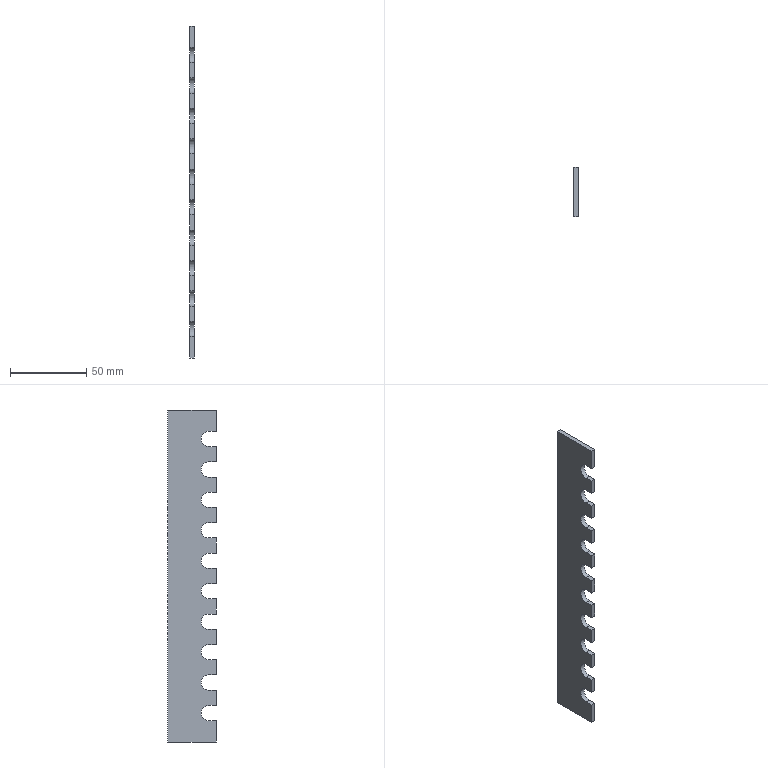Part | SolidWorks | features ExtruThin 1, ICE 1, LPattern 1 | 1 solid | 46 faces | box 3 x 32 x 218 mm | volume 18250 mm3 | plane 36 | cylinder 10 | commonest cylinder face diameters 10 x10
STEP:
#1=CARTESIAN_POINT('',(-3.,-32.,14.));
#2=VERTEX_POINT('',#1);
#3=CARTESIAN_POINT('',(0.,-32.,14.));
#4=VERTEX_POINT('',#3);
#5=CARTESIAN_POINT('',(-3.,-32.,14.));
#6=DIRECTION('',(1.,0.,0.));
#7=VECTOR('',#6,1000.);
#8=LINE('',#5,#7);
#9=EDGE_CURVE('',#2,#4,#8,.T.);
#10=ORIENTED_EDGE('',*,*,#9,.F.);
#11=CARTESIAN_POINT('',(-3.,-32.,0.));
#12=VERTEX_POINT('',#11);
#13=CARTESIAN_POINT('',(-3.,-32.,218.));
#14=DIRECTION('',(0.,0.,-1.));
#15=VECTOR('',#14,1000.);
#16=LINE('',#13,#15);
#17=EDGE_CURVE('',#2,#12,#16,.T.);
#18=ORIENTED_EDGE('',*,*,#17,.T.);
#19=CARTESIAN_POINT('',(0.,-32.,0.));
#20=VERTEX_POINT('',#19);
#21=CARTESIAN_POINT('',(0.,-32.,0.));
#22=DIRECTION('',(-1.,0.,0.));
#23=VECTOR('',#22,1000.);
#24=LINE('',#21,#23);
#25=EDGE_CURVE('',#20,#12,#24,.T.);
#26=ORIENTED_EDGE('',*,*,#25,.F.);
#27=CARTESIAN_POINT('',(0.,-32.,218.));
#28=DIRECTION('',(0.,0.,-1.));
#29=VECTOR('',#28,1000.);
#30=LINE('',#27,#29);
#31=EDGE_CURVE('',#4,#20,#30,.T.);
#32=ORIENTED_EDGE('',*,*,#31,.F.);
#33=EDGE_LOOP('',(#10,#18,#26,#32));
#34=FACE_OUTER_BOUND('',#33,.T.);
#35=CARTESIAN_POINT('',(0.,-32.,218.));
#36=DIRECTION('',(0.,-1.,0.));
#37=DIRECTION('',(0.,0.,-1.));
#38=AXIS2_PLACEMENT_3D('',#35,#36,#37);
#39=PLANE('',#38);
#40=ADVANCED_FACE('',(#34),#39,.T.);
#41=CARTESIAN_POINT('',(-3.,-32.,24.));
#42=VERTEX_POINT('',#41);
#43=CARTESIAN_POINT('',(0.,-32.,24.));
#44=VERTEX_POINT('',#43);
#45=CARTESIAN_POINT('',(-3.,-32.,24.));
#46=DIRECTION('',(1.,0.,0.));
#47=VECTOR('',#46,1000.);
#48=LINE('',#45,#47);
#49=EDGE_CURVE('',#42,#44,#48,.T.);
#50=ORIENTED_EDGE('',*,*,#49,.T.);
#51=CARTESIAN_POINT('',(0.,-32.,34.));
#52=VERTEX_POINT('',#51);
#53=CARTESIAN_POINT('',(0.,-32.,218.));
#54=DIRECTION('',(0.,0.,-1.));
#55=VECTOR('',#54,1000.);
#56=LINE('',#53,#55);
#57=EDGE_CURVE('',#52,#44,#56,.T.);
#58=ORIENTED_EDGE('',*,*,#57,.F.);
#59=CARTESIAN_POINT('',(-3.,-32.,34.));
#60=VERTEX_POINT('',#59);
#61=CARTESIAN_POINT('',(-3.,-32.,34.));
#62=DIRECTION('',(1.,0.,0.));
#63=VECTOR('',#62,1000.);
#64=LINE('',#61,#63);
#65=EDGE_CURVE('',#60,#52,#64,.T.);
#66=ORIENTED_EDGE('',*,*,#65,.F.);
#67=CARTESIAN_POINT('',(-3.,-32.,218.));
#68=DIRECTION('',(0.,0.,-1.));
#69=VECTOR('',#68,1000.);
#70=LINE('',#67,#69);
#71=EDGE_CURVE('',#60,#42,#70,.T.);
#72=ORIENTED_EDGE('',*,*,#71,.T.);
#73=EDGE_LOOP('',(#50,#58,#66,#72));
#74=FACE_OUTER_BOUND('',#73,.T.);
#75=CARTESIAN_POINT('',(0.,-32.,218.));
#76=DIRECTION('',(0.,-1.,0.));
#77=DIRECTION('',(0.,0.,-1.));
#78=AXIS2_PLACEMENT_3D('',#75,#76,#77);
#79=PLANE('',#78);
#80=ADVANCED_FACE('',(#74),#79,.T.);
#81=CARTESIAN_POINT('',(-3.,-32.,44.));
#82=VERTEX_POINT('',#81);
#83=CARTESIAN_POINT('',(0.,-32.,44.));
#84=VERTEX_POINT('',#83);
#85=CARTESIAN_POINT('',(-3.,-32.,44.));
#86=DIRECTION('',(1.,0.,0.));
#87=VECTOR('',#86,1000.);
#88=LINE('',#85,#87);
#89=EDGE_CURVE('',#82,#84,#88,.T.);
#90=ORIENTED_EDGE('',*,*,#89,.T.);
#91=CARTESIAN_POINT('',(0.,-32.,54.));
#92=VERTEX_POINT('',#91);
#93=CARTESIAN_POINT('',(0.,-32.,218.));
#94=DIRECTION('',(0.,0.,-1.));
#95=VECTOR('',#94,1000.);
#96=LINE('',#93,#95);
#97=EDGE_CURVE('',#92,#84,#96,.T.);
#98=ORIENTED_EDGE('',*,*,#97,.F.);
#99=CARTESIAN_POINT('',(-3.,-32.,54.));
#100=VERTEX_POINT('',#99);
#101=CARTESIAN_POINT('',(-3.,-32.,54.));
#102=DIRECTION('',(1.,0.,0.));
#103=VECTOR('',#102,1000.);
#104=LINE('',#101,#103);
#105=EDGE_CURVE('',#100,#92,#104,.T.);
#106=ORIENTED_EDGE('',*,*,#105,.F.);
#107=CARTESIAN_POINT('',(-3.,-32.,218.));
#108=DIRECTION('',(0.,0.,-1.));
#109=VECTOR('',#108,1000.);
#110=LINE('',#107,#109);
#111=EDGE_CURVE('',#100,#82,#110,.T.);
#112=ORIENTED_EDGE('',*,*,#111,.T.);
#113=EDGE_LOOP('',(#90,#98,#106,#112));
#114=FACE_OUTER_BOUND('',#113,.T.);
#115=CARTESIAN_POINT('',(0.,-32.,218.));
#116=DIRECTION('',(0.,-1.,0.));
#117=DIRECTION('',(0.,0.,-1.));
#118=AXIS2_PLACEMENT_3D('',#115,#116,#117);
#119=PLANE('',#118);
#120=ADVANCED_FACE('',(#114),#119,.T.);
#121=CARTESIAN_POINT('',(-3.,-32.,64.));
#122=VERTEX_POINT('',#121);
#123=CARTESIAN_POINT('',(0.,-32.,64.));
#124=VERTEX_POINT('',#123);
#125=CARTESIAN_POINT('',(-3.,-32.,64.));
#126=DIRECTION('',(1.,0.,0.));
#127=VECTOR('',#126,1000.);
#128=LINE('',#125,#127);
#129=EDGE_CURVE('',#122,#124,#128,.T.);
#130=ORIENTED_EDGE('',*,*,#129,.T.);
#131=CARTESIAN_POINT('',(0.,-32.,74.));
#132=VERTEX_POINT('',#131);
#133=CARTESIAN_POINT('',(0.,-32.,218.));
#134=DIRECTION('',(0.,0.,-1.));
#135=VECTOR('',#134,1000.);
#136=LINE('',#133,#135);
#137=EDGE_CURVE('',#132,#124,#136,.T.);
#138=ORIENTED_EDGE('',*,*,#137,.F.);
#139=CARTESIAN_POINT('',(-3.,-32.,74.));
#140=VERTEX_POINT('',#139);
#141=CARTESIAN_POINT('',(-3.,-32.,74.));
#142=DIRECTION('',(1.,0.,0.));
#143=VECTOR('',#142,1000.);
#144=LINE('',#141,#143);
#145=EDGE_CURVE('',#140,#132,#144,.T.);
#146=ORIENTED_EDGE('',*,*,#145,.F.);
#147=CARTESIAN_POINT('',(-3.,-32.,218.));
#148=DIRECTION('',(0.,0.,-1.));
#149=VECTOR('',#148,1000.);
#150=LINE('',#147,#149);
#151=EDGE_CURVE('',#140,#122,#150,.T.);
#152=ORIENTED_EDGE('',*,*,#151,.T.);
#153=EDGE_LOOP('',(#130,#138,#146,#152));
#154=FACE_OUTER_BOUND('',#153,.T.);
#155=CARTESIAN_POINT('',(0.,-32.,218.));
#156=DIRECTION('',(0.,-1.,0.));
#157=DIRECTION('',(0.,0.,-1.));
#158=AXIS2_PLACEMENT_3D('',#155,#156,#157);
#159=PLANE('',#158);
#160=ADVANCED_FACE('',(#154),#159,.T.);
#161=CARTESIAN_POINT('',(-3.,-32.,84.));
#162=VERTEX_POINT('',#161);
#163=CARTESIAN_POINT('',(0.,-32.,84.));
#164=VERTEX_POINT('',#163);
#165=CARTESIAN_POINT('',(-3.,-32.,84.));
#166=DIRECTION('',(1.,0.,0.));
#167=VECTOR('',#166,1000.);
#168=LINE('',#165,#167);
#169=EDGE_CURVE('',#162,#164,#168,.T.);
#170=ORIENTED_EDGE('',*,*,#169,.T.);
#171=CARTESIAN_POINT('',(0.,-32.,94.));
#172=VERTEX_POINT('',#171);
#173=CARTESIAN_POINT('',(0.,-32.,218.));
#174=DIRECTION('',(0.,0.,-1.));
#175=VECTOR('',#174,1000.);
#176=LINE('',#173,#175);
#177=EDGE_CURVE('',#172,#164,#176,.T.);
#178=ORIENTED_EDGE('',*,*,#177,.F.);
#179=CARTESIAN_POINT('',(-3.,-32.,94.));
#180=VERTEX_POINT('',#179);
#181=CARTESIAN_POINT('',(-3.,-32.,94.));
#182=DIRECTION('',(1.,0.,0.));
#183=VECTOR('',#182,1000.);
#184=LINE('',#181,#183);
#185=EDGE_CURVE('',#180,#172,#184,.T.);
#186=ORIENTED_EDGE('',*,*,#185,.F.);
#187=CARTESIAN_POINT('',(-3.,-32.,218.));
#188=DIRECTION('',(0.,0.,-1.));
#189=VECTOR('',#188,1000.);
#190=LINE('',#187,#189);
#191=EDGE_CURVE('',#180,#162,#190,.T.);
#192=ORIENTED_EDGE('',*,*,#191,.T.);
#193=EDGE_LOOP('',(#170,#178,#186,#192));
#194=FACE_OUTER_BOUND('',#193,.T.);
#195=CARTESIAN_POINT('',(0.,-32.,218.));
#196=DIRECTION('',(0.,-1.,0.));
#197=DIRECTION('',(0.,0.,-1.));
#198=AXIS2_PLACEMENT_3D('',#195,#196,#197);
#199=PLANE('',#198);
#200=ADVANCED_FACE('',(#194),#199,.T.);
#201=CARTESIAN_POINT('',(-3.,-32.,104.));
#202=VERTEX_POINT('',#201);
#203=CARTESIAN_POINT('',(0.,-32.,104.));
#204=VERTEX_POINT('',#203);
#205=CARTESIAN_POINT('',(-3.,-32.,104.));
#206=DIRECTION('',(1.,0.,0.));
#207=VECTOR('',#206,1000.);
#208=LINE('',#205,#207);
#209=EDGE_CURVE('',#202,#204,#208,.T.);
#210=ORIENTED_EDGE('',*,*,#209,.T.);
#211=CARTESIAN_POINT('',(0.,-32.,114.));
#212=VERTEX_POINT('',#211);
#213=CARTESIAN_POINT('',(0.,-32.,218.));
#214=DIRECTION('',(0.,0.,-1.));
#215=VECTOR('',#214,1000.);
#216=LINE('',#213,#215);
#217=EDGE_CURVE('',#212,#204,#216,.T.);
#218=ORIENTED_EDGE('',*,*,#217,.F.);
#219=CARTESIAN_POINT('',(-3.,-32.,114.));
#220=VERTEX_POINT('',#219);
#221=CARTESIAN_POINT('',(-3.,-32.,114.));
#222=DIRECTION('',(1.,0.,0.));
#223=VECTOR('',#222,1000.);
#224=LINE('',#221,#223);
#225=EDGE_CURVE('',#220,#212,#224,.T.);
#226=ORIENTED_EDGE('',*,*,#225,.F.);
#227=CARTESIAN_POINT('',(-3.,-32.,218.));
#228=DIRECTION('',(0.,0.,-1.));
#229=VECTOR('',#228,1000.);
#230=LINE('',#227,#229);
#231=EDGE_CURVE('',#220,#202,#230,.T.);
#232=ORIENTED_EDGE('',*,*,#231,.T.);
#233=EDGE_LOOP('',(#210,#218,#226,#232));
#234=FACE_OUTER_BOUND('',#233,.T.);
#235=CARTESIAN_POINT('',(0.,-32.,218.));
#236=DIRECTION('',(0.,-1.,0.));
#237=DIRECTION('',(0.,0.,-1.));
#238=AXIS2_PLACEMENT_3D('',#235,#236,#237);
#239=PLANE('',#238);
#240=ADVANCED_FACE('',(#234),#239,.T.);
#241=CARTESIAN_POINT('',(-3.,-32.,124.));
#242=VERTEX_POINT('',#241);
#243=CARTESIAN_POINT('',(0.,-32.,124.));
#244=VERTEX_POINT('',#243);
#245=CARTESIAN_POINT('',(-3.,-32.,124.));
#246=DIRECTION('',(1.,0.,0.));
#247=VECTOR('',#246,1000.);
#248=LINE('',#245,#247);
#249=EDGE_CURVE('',#242,#244,#248,.T.);
#250=ORIENTED_EDGE('',*,*,#249,.T.);
#251=CARTESIAN_POINT('',(0.,-32.,134.));
#252=VERTEX_POINT('',#251);
#253=CARTESIAN_POINT('',(0.,-32.,218.));
#254=DIRECTION('',(0.,0.,-1.));
#255=VECTOR('',#254,1000.);
#256=LINE('',#253,#255);
#257=EDGE_CURVE('',#252,#244,#256,.T.);
#258=ORIENTED_EDGE('',*,*,#257,.F.);
#259=CARTESIAN_POINT('',(-3.,-32.,134.));
#260=VERTEX_POINT('',#259);
#261=CARTESIAN_POINT('',(-3.,-32.,134.));
#262=DIRECTION('',(1.,0.,0.));
#263=VECTOR('',#262,1000.);
#264=LINE('',#261,#263);
#265=EDGE_CURVE('',#260,#252,#264,.T.);
#266=ORIENTED_EDGE('',*,*,#265,.F.);
#267=CARTESIAN_POINT('',(-3.,-32.,218.));
#268=DIRECTION('',(0.,0.,-1.));
#269=VECTOR('',#268,1000.);
#270=LINE('',#267,#269);
#271=EDGE_CURVE('',#260,#242,#270,.T.);
#272=ORIENTED_EDGE('',*,*,#271,.T.);
#273=EDGE_LOOP('',(#250,#258,#266,#272));
#274=FACE_OUTER_BOUND('',#273,.T.);
#275=CARTESIAN_POINT('',(0.,-32.,218.));
#276=DIRECTION('',(0.,-1.,0.));
#277=DIRECTION('',(0.,0.,-1.));
#278=AXIS2_PLACEMENT_3D('',#275,#276,#277);
#279=PLANE('',#278);
#280=ADVANCED_FACE('',(#274),#279,.T.);
#281=CARTESIAN_POINT('',(-3.,-32.,144.));
#282=VERTEX_POINT('',#281);
#283=CARTESIAN_POINT('',(0.,-32.,144.));
#284=VERTEX_POINT('',#283);
#285=CARTESIAN_POINT('',(-3.,-32.,144.));
#286=DIRECTION('',(1.,0.,0.));
#287=VECTOR('',#286,1000.);
#288=LINE('',#285,#287);
#289=EDGE_CURVE('',#282,#284,#288,.T.);
#290=ORIENTED_EDGE('',*,*,#289,.T.);
#291=CARTESIAN_POINT('',(0.,-32.,154.));
#292=VERTEX_POINT('',#291);
#293=CARTESIAN_POINT('',(0.,-32.,218.));
#294=DIRECTION('',(0.,0.,-1.));
#295=VECTOR('',#294,1000.);
#296=LINE('',#293,#295);
#297=EDGE_CURVE('',#292,#284,#296,.T.);
#298=ORIENTED_EDGE('',*,*,#297,.F.);
#299=CARTESIAN_POINT('',(-3.,-32.,154.));
#300=VERTEX_POINT('',#299);
#301=CARTESIAN_POINT('',(-3.,-32.,154.));
#302=DIRECTION('',(1.,0.,0.));
#303=VECTOR('',#302,1000.);
#304=LINE('',#301,#303);
#305=EDGE_CURVE('',#300,#292,#304,.T.);
#306=ORIENTED_EDGE('',*,*,#305,.F.);
#307=CARTESIAN_POINT('',(-3.,-32.,218.));
#308=DIRECTION('',(0.,0.,-1.));
#309=VECTOR('',#308,1000.);
#310=LINE('',#307,#309);
#311=EDGE_CURVE('',#300,#282,#310,.T.);
#312=ORIENTED_EDGE('',*,*,#311,.T.);
#313=EDGE_LOOP('',(#290,#298,#306,#312));
#314=FACE_OUTER_BOUND('',#313,.T.);
#315=CARTESIAN_POINT('',(0.,-32.,218.));
#316=DIRECTION('',(0.,-1.,0.));
#317=DIRECTION('',(0.,0.,-1.));
#318=AXIS2_PLACEMENT_3D('',#315,#316,#317);
#319=PLANE('',#318);
#320=ADVANCED_FACE('',(#314),#319,.T.);
#321=CARTESIAN_POINT('',(-3.,-32.,164.));
#322=VERTEX_POINT('',#321);
#323=CARTESIAN_POINT('',(0.,-32.,164.));
#324=VERTEX_POINT('',#323);
#325=CARTESIAN_POINT('',(-3.,-32.,164.));
#326=DIRECTION('',(1.,0.,0.));
#327=VECTOR('',#326,1000.);
#328=LINE('',#325,#327);
#329=EDGE_CURVE('',#322,#324,#328,.T.);
#330=ORIENTED_EDGE('',*,*,#329,.T.);
#331=CARTESIAN_POINT('',(0.,-32.,174.));
#332=VERTEX_POINT('',#331);
#333=CARTESIAN_POINT('',(0.,-32.,218.));
#334=DIRECTION('',(0.,0.,-1.));
#335=VECTOR('',#334,1000.);
#336=LINE('',#333,#335);
#337=EDGE_CURVE('',#332,#324,#336,.T.);
#338=ORIENTED_EDGE('',*,*,#337,.F.);
#339=CARTESIAN_POINT('',(-3.,-32.,174.));
#340=VERTEX_POINT('',#339);
#341=CARTESIAN_POINT('',(-3.,-32.,174.));
#342=DIRECTION('',(1.,0.,0.));
#343=VECTOR('',#342,1000.);
#344=LINE('',#341,#343);
#345=EDGE_CURVE('',#340,#332,#344,.T.);
#346=ORIENTED_EDGE('',*,*,#345,.F.);
#347=CARTESIAN_POINT('',(-3.,-32.,218.));
#348=DIRECTION('',(0.,0.,-1.));
#349=VECTOR('',#348,1000.);
#350=LINE('',#347,#349);
#351=EDGE_CURVE('',#340,#322,#350,.T.);
#352=ORIENTED_EDGE('',*,*,#351,.T.);
#353=EDGE_LOOP('',(#330,#338,#346,#352));
#354=FACE_OUTER_BOUND('',#353,.T.);
#355=CARTESIAN_POINT('',(0.,-32.,218.));
#356=DIRECTION('',(0.,-1.,0.));
#357=DIRECTION('',(0.,0.,-1.));
#358=AXIS2_PLACEMENT_3D('',#355,#356,#357);
#359=PLANE('',#358);
#360=ADVANCED_FACE('',(#354),#359,.T.);
#361=CARTESIAN_POINT('',(-3.,-32.,184.));
#362=VERTEX_POINT('',#361);
#363=CARTESIAN_POINT('',(0.,-32.,184.));
#364=VERTEX_POINT('',#363);
#365=CARTESIAN_POINT('',(-3.,-32.,184.));
#366=DIRECTION('',(1.,0.,0.));
#367=VECTOR('',#366,1000.);
#368=LINE('',#365,#367);
#369=EDGE_CURVE('',#362,#364,#368,.T.);
#370=ORIENTED_EDGE('',*,*,#369,.T.);
#371=CARTESIAN_POINT('',(0.,-32.,194.));
#372=VERTEX_POINT('',#371);
#373=CARTESIAN_POINT('',(0.,-32.,218.));
#374=DIRECTION('',(0.,0.,-1.));
#375=VECTOR('',#374,1000.);
#376=LINE('',#373,#375);
#377=EDGE_CURVE('',#372,#364,#376,.T.);
#378=ORIENTED_EDGE('',*,*,#377,.F.);
#379=CARTESIAN_POINT('',(-3.,-32.,194.));
#380=VERTEX_POINT('',#379);
#381=CARTESIAN_POINT('',(-3.,-32.,194.));
#382=DIRECTION('',(1.,0.,0.));
#383=VECTOR('',#382,1000.);
#384=LINE('',#381,#383);
#385=EDGE_CURVE('',#380,#372,#384,.T.);
#386=ORIENTED_EDGE('',*,*,#385,.F.);
#387=CARTESIAN_POINT('',(-3.,-32.,218.));
#388=DIRECTION('',(0.,0.,-1.));
#389=VECTOR('',#388,1000.);
#390=LINE('',#387,#389);
#391=EDGE_CURVE('',#380,#362,#390,.T.);
#392=ORIENTED_EDGE('',*,*,#391,.T.);
#393=EDGE_LOOP('',(#370,#378,#386,#392));
#394=FACE_OUTER_BOUND('',#393,.T.);
#395=CARTESIAN_POINT('',(0.,-32.,218.));
#396=DIRECTION('',(0.,-1.,0.));
#397=DIRECTION('',(0.,0.,-1.));
#398=AXIS2_PLACEMENT_3D('',#395,#396,#397);
#399=PLANE('',#398);
#400=ADVANCED_FACE('',(#394),#399,.T.);
#401=ORIENTED_EDGE('',*,*,#17,.F.);
#402=CARTESIAN_POINT('',(-3.,-27.,14.));
#403=VERTEX_POINT('',#402);
#404=CARTESIAN_POINT('',(-3.,-27.,14.));
#405=DIRECTION('',(0.,1.,0.));
#406=VECTOR('',#405,1000.);
#407=LINE('',#404,#406);
#408=EDGE_CURVE('',#2,#403,#407,.T.);
#409=ORIENTED_EDGE('',*,*,#408,.T.);
#410=CARTESIAN_POINT('',(-3.,-27.,24.));
#411=VERTEX_POINT('',#410);
#412=CARTESIAN_POINT('',(-3.,-27.,19.));
#413=DIRECTION('',(1.,0.,0.));
#414=DIRECTION('',(0.,0.,-1.));
#415=AXIS2_PLACEMENT_3D('',#412,#413,#414);
#416=CIRCLE('',#415,5.);
#417=EDGE_CURVE('',#403,#411,#416,.T.);
#418=ORIENTED_EDGE('',*,*,#417,.T.);
#419=CARTESIAN_POINT('',(-3.,-32.,24.));
#420=DIRECTION('',(0.,-1.,0.));
#421=VECTOR('',#420,1000.);
#422=LINE('',#419,#421);
#423=EDGE_CURVE('',#411,#42,#422,.T.);
#424=ORIENTED_EDGE('',*,*,#423,.T.);
#425=ORIENTED_EDGE('',*,*,#71,.F.);
#426=CARTESIAN_POINT('',(-3.,-27.,34.));
#427=VERTEX_POINT('',#426);
#428=CARTESIAN_POINT('',(-3.,-27.,34.));
#429=DIRECTION('',(0.,1.,0.));
#430=VECTOR('',#429,1000.);
#431=LINE('',#428,#430);
#432=EDGE_CURVE('',#60,#427,#431,.T.);
#433=ORIENTED_EDGE('',*,*,#432,.T.);
#434=CARTESIAN_POINT('',(-3.,-27.,44.));
#435=VERTEX_POINT('',#434);
#436=CARTESIAN_POINT('',(-3.,-27.,39.));
#437=DIRECTION('',(1.,0.,0.));
#438=DIRECTION('',(0.,0.,-1.));
#439=AXIS2_PLACEMENT_3D('',#436,#437,#438);
#440=CIRCLE('',#439,5.);
#441=EDGE_CURVE('',#427,#435,#440,.T.);
#442=ORIENTED_EDGE('',*,*,#441,.T.);
#443=CARTESIAN_POINT('',(-3.,-32.,44.));
#444=DIRECTION('',(0.,-1.,0.));
#445=VECTOR('',#444,1000.);
#446=LINE('',#443,#445);
#447=EDGE_CURVE('',#435,#82,#446,.T.);
#448=ORIENTED_EDGE('',*,*,#447,.T.);
#449=ORIENTED_EDGE('',*,*,#111,.F.);
#450=CARTESIAN_POINT('',(-3.,-27.,54.));
#451=VERTEX_POINT('',#450);
#452=CARTESIAN_POINT('',(-3.,-27.,54.));
#453=DIRECTION('',(0.,1.,0.));
#454=VECTOR('',#453,1000.);
#455=LINE('',#452,#454);
#456=EDGE_CURVE('',#100,#451,#455,.T.);
#457=ORIENTED_EDGE('',*,*,#456,.T.);
#458=CARTESIAN_POINT('',(-3.,-27.,64.));
#459=VERTEX_POINT('',#458);
#460=CARTESIAN_POINT('',(-3.,-27.,59.));
#461=DIRECTION('',(1.,0.,0.));
#462=DIRECTION('',(0.,0.,-1.));
#463=AXIS2_PLACEMENT_3D('',#460,#461,#462);
#464=CIRCLE('',#463,5.);
#465=EDGE_CURVE('',#451,#459,#464,.T.);
#466=ORIENTED_EDGE('',*,*,#465,.T.);
#467=CARTESIAN_POINT('',(-3.,-32.,64.));
#468=DIRECTION('',(0.,-1.,0.));
#469=VECTOR('',#468,1000.);
#470=LINE('',#467,#469);
#471=EDGE_CURVE('',#459,#122,#470,.T.);
#472=ORIENTED_EDGE('',*,*,#471,.T.);
#473=ORIENTED_EDGE('',*,*,#151,.F.);
#474=CARTESIAN_POINT('',(-3.,-27.,74.));
#475=VERTEX_POINT('',#474);
#476=CARTESIAN_POINT('',(-3.,-27.,74.));
#477=DIRECTION('',(0.,1.,0.));
#478=VECTOR('',#477,1000.);
#479=LINE('',#476,#478);
#480=EDGE_CURVE('',#140,#475,#479,.T.);
#481=ORIENTED_EDGE('',*,*,#480,.T.);
#482=CARTESIAN_POINT('',(-3.,-27.,84.));
#483=VERTEX_POINT('',#482);
#484=CARTESIAN_POINT('',(-3.,-27.,79.));
#485=DIRECTION('',(1.,0.,0.));
#486=DIRECTION('',(0.,0.,-1.));
#487=AXIS2_PLACEMENT_3D('',#484,#485,#486);
#488=CIRCLE('',#487,5.);
#489=EDGE_CURVE('',#475,#483,#488,.T.);
#490=ORIENTED_EDGE('',*,*,#489,.T.);
#491=CARTESIAN_POINT('',(-3.,-32.,84.));
#492=DIRECTION('',(0.,-1.,0.));
#493=VECTOR('',#492,1000.);
#494=LINE('',#491,#493);
#495=EDGE_CURVE('',#483,#162,#494,.T.);
#496=ORIENTED_EDGE('',*,*,#495,.T.);
#497=ORIENTED_EDGE('',*,*,#191,.F.);
#498=CARTESIAN_POINT('',(-3.,-27.,94.));
#499=VERTEX_POINT('',#498);
#500=CARTESIAN_POINT('',(-3.,-27.,94.));
#501=DIRECTION('',(0.,1.,0.));
#502=VECTOR('',#501,1000.);
#503=LINE('',#500,#502);
#504=EDGE_CURVE('',#180,#499,#503,.T.);
#505=ORIENTED_EDGE('',*,*,#504,.T.);
#506=CARTESIAN_POINT('',(-3.,-27.,104.));
#507=VERTEX_POINT('',#506);
#508=CARTESIAN_POINT('',(-3.,-27.,99.));
#509=DIRECTION('',(1.,0.,0.));
#510=DIRECTION('',(0.,0.,-1.));
#511=AXIS2_PLACEMENT_3D('',#508,#509,#510);
#512=CIRCLE('',#511,5.);
#513=EDGE_CURVE('',#499,#507,#512,.T.);
#514=ORIENTED_EDGE('',*,*,#513,.T.);
#515=CARTESIAN_POINT('',(-3.,-32.,104.));
#516=DIRECTION('',(0.,-1.,0.));
#517=VECTOR('',#516,1000.);
#518=LINE('',#515,#517);
#519=EDGE_CURVE('',#507,#202,#518,.T.);
#520=ORIENTED_EDGE('',*,*,#519,.T.);
#521=ORIENTED_EDGE('',*,*,#231,.F.);
#522=CARTESIAN_POINT('',(-3.,-27.,114.));
#523=VERTEX_POINT('',#522);
#524=CARTESIAN_POINT('',(-3.,-27.,114.));
#525=DIRECTION('',(0.,1.,0.));
#526=VECTOR('',#525,1000.);
#527=LINE('',#524,#526);
#528=EDGE_CURVE('',#220,#523,#527,.T.);
#529=ORIENTED_EDGE('',*,*,#528,.T.);
#530=CARTESIAN_POINT('',(-3.,-27.,124.));
#531=VERTEX_POINT('',#530);
#532=CARTESIAN_POINT('',(-3.,-27.,119.));
#533=DIRECTION('',(1.,0.,0.));
#534=DIRECTION('',(0.,0.,-1.));
#535=AXIS2_PLACEMENT_3D('',#532,#533,#534);
#536=CIRCLE('',#535,5.);
#537=EDGE_CURVE('',#523,#531,#536,.T.);
#538=ORIENTED_EDGE('',*,*,#537,.T.);
#539=CARTESIAN_POINT('',(-3.,-32.,124.));
#540=DIRECTION('',(0.,-1.,0.));
#541=VECTOR('',#540,1000.);
#542=LINE('',#539,#541);
#543=EDGE_CURVE('',#531,#242,#542,.T.);
#544=ORIENTED_EDGE('',*,*,#543,.T.);
#545=ORIENTED_EDGE('',*,*,#271,.F.);
#546=CARTESIAN_POINT('',(-3.,-27.,134.));
#547=VERTEX_POINT('',#546);
#548=CARTESIAN_POINT('',(-3.,-27.,134.));
#549=DIRECTION('',(0.,1.,0.));
#550=VECTOR('',#549,1000.);
#551=LINE('',#548,#550);
#552=EDGE_CURVE('',#260,#547,#551,.T.);
#553=ORIENTED_EDGE('',*,*,#552,.T.);
#554=CARTESIAN_POINT('',(-3.,-27.,144.));
#555=VERTEX_POINT('',#554);
#556=CARTESIAN_POINT('',(-3.,-27.,139.));
#557=DIRECTION('',(1.,0.,0.));
#558=DIRECTION('',(0.,0.,-1.));
#559=AXIS2_PLACEMENT_3D('',#556,#557,#558);
#560=CIRCLE('',#559,5.);
#561=EDGE_CURVE('',#547,#555,#560,.T.);
#562=ORIENTED_EDGE('',*,*,#561,.T.);
#563=CARTESIAN_POINT('',(-3.,-32.,144.));
#564=DIRECTION('',(0.,-1.,0.));
#565=VECTOR('',#564,1000.);
#566=LINE('',#563,#565);
#567=EDGE_CURVE('',#555,#282,#566,.T.);
#568=ORIENTED_EDGE('',*,*,#567,.T.);
#569=ORIENTED_EDGE('',*,*,#311,.F.);
#570=CARTESIAN_POINT('',(-3.,-27.,154.));
#571=VERTEX_POINT('',#570);
#572=CARTESIAN_POINT('',(-3.,-27.,154.));
#573=DIRECTION('',(0.,1.,0.));
#574=VECTOR('',#573,1000.);
#575=LINE('',#572,#574);
#576=EDGE_CURVE('',#300,#571,#575,.T.);
#577=ORIENTED_EDGE('',*,*,#576,.T.);
#578=CARTESIAN_POINT('',(-3.,-27.,164.));
#579=VERTEX_POINT('',#578);
#580=CARTESIAN_POINT('',(-3.,-27.,159.));
#581=DIRECTION('',(1.,0.,0.));
#582=DIRECTION('',(0.,0.,-1.));
#583=AXIS2_PLACEMENT_3D('',#580,#581,#582);
#584=CIRCLE('',#583,5.);
#585=EDGE_CURVE('',#571,#579,#584,.T.);
#586=ORIENTED_EDGE('',*,*,#585,.T.);
#587=CARTESIAN_POINT('',(-3.,-32.,164.));
#588=DIRECTION('',(0.,-1.,0.));
#589=VECTOR('',#588,1000.);
#590=LINE('',#587,#589);
#591=EDGE_CURVE('',#579,#322,#590,.T.);
#592=ORIENTED_EDGE('',*,*,#591,.T.);
#593=ORIENTED_EDGE('',*,*,#351,.F.);
#594=CARTESIAN_POINT('',(-3.,-27.,174.));
#595=VERTEX_POINT('',#594);
#596=CARTESIAN_POINT('',(-3.,-27.,174.));
#597=DIRECTION('',(0.,1.,0.));
#598=VECTOR('',#597,1000.);
#599=LINE('',#596,#598);
#600=EDGE_CURVE('',#340,#595,#599,.T.);
#601=ORIENTED_EDGE('',*,*,#600,.T.);
#602=CARTESIAN_POINT('',(-3.,-27.,184.));
#603=VERTEX_POINT('',#602);
#604=CARTESIAN_POINT('',(-3.,-27.,179.));
#605=DIRECTION('',(1.,0.,0.));
#606=DIRECTION('',(0.,0.,-1.));
#607=AXIS2_PLACEMENT_3D('',#604,#605,#606);
#608=CIRCLE('',#607,5.);
#609=EDGE_CURVE('',#595,#603,#608,.T.);
#610=ORIENTED_EDGE('',*,*,#609,.T.);
#611=CARTESIAN_POINT('',(-3.,-32.,184.));
#612=DIRECTION('',(0.,-1.,0.));
#613=VECTOR('',#612,1000.);
#614=LINE('',#611,#613);
#615=EDGE_CURVE('',#603,#362,#614,.T.);
#616=ORIENTED_EDGE('',*,*,#615,.T.);
#617=ORIENTED_EDGE('',*,*,#391,.F.);
#618=CARTESIAN_POINT('',(-3.,-27.,194.));
#619=VERTEX_POINT('',#618);
#620=CARTESIAN_POINT('',(-3.,-27.,194.));
#621=DIRECTION('',(0.,1.,0.));
#622=VECTOR('',#621,1000.);
#623=LINE('',#620,#622);
#624=EDGE_CURVE('',#380,#619,#623,.T.);
#625=ORIENTED_EDGE('',*,*,#624,.T.);
#626=CARTESIAN_POINT('',(-3.,-27.,204.));
#627=VERTEX_POINT('',#626);
#628=CARTESIAN_POINT('',(-3.,-27.,199.));
#629=DIRECTION('',(1.,0.,0.));
#630=DIRECTION('',(0.,0.,-1.));
#631=AXIS2_PLACEMENT_3D('',#628,#629,#630);
#632=CIRCLE('',#631,5.);
#633=EDGE_CURVE('',#619,#627,#632,.T.);
#634=ORIENTED_EDGE('',*,*,#633,.T.);
#635=CARTESIAN_POINT('',(-3.,-32.,204.));
#636=VERTEX_POINT('',#635);
#637=CARTESIAN_POINT('',(-3.,-32.,204.));
#638=DIRECTION('',(0.,-1.,0.));
#639=VECTOR('',#638,1000.);
#640=LINE('',#637,#639);
#641=EDGE_CURVE('',#627,#636,#640,.T.);
#642=ORIENTED_EDGE('',*,*,#641,.T.);
#643=CARTESIAN_POINT('',(-3.,-32.,218.));
#644=VERTEX_POINT('',#643);
#645=CARTESIAN_POINT('',(-3.,-32.,218.));
#646=DIRECTION('',(0.,0.,-1.));
#647=VECTOR('',#646,1000.);
#648=LINE('',#645,#647);
#649=EDGE_CURVE('',#644,#636,#648,.T.);
#650=ORIENTED_EDGE('',*,*,#649,.F.);
#651=CARTESIAN_POINT('',(-3.,0.,218.));
#652=VERTEX_POINT('',#651);
#653=CARTESIAN_POINT('',(-3.,0.,218.));
#654=DIRECTION('',(0.,-1.,0.));
#655=VECTOR('',#654,1000.);
#656=LINE('',#653,#655);
#657=EDGE_CURVE('',#652,#644,#656,.T.);
#658=ORIENTED_EDGE('',*,*,#657,.F.);
#659=CARTESIAN_POINT('',(-3.,0.,0.));
#660=VERTEX_POINT('',#659);
#661=CARTESIAN_POINT('',(-3.,0.,218.));
#662=DIRECTION('',(0.,0.,-1.));
#663=VECTOR('',#662,1000.);
#664=LINE('',#661,#663);
#665=EDGE_CURVE('',#652,#660,#664,.T.);
#666=ORIENTED_EDGE('',*,*,#665,.T.);
#667=CARTESIAN_POINT('',(-3.,0.,0.));
#668=DIRECTION('',(0.,-1.,0.));
#669=VECTOR('',#668,1000.);
#670=LINE('',#667,#669);
#671=EDGE_CURVE('',#660,#12,#670,.T.);
#672=ORIENTED_EDGE('',*,*,#671,.T.);
#673=EDGE_LOOP('',(#401,#409,#418,#424,#425,#433,#442,#448,#449,#457,#466,#472,#473,#481,#490,#496,#497,#505,#514,#520,#521,#529,#538,#544,#545,#553,#562,#568,#569,#577,#586,#592,#593,#601,#610,#616,#617,#625,#634,#642,#650,#658,#666,#672));
#674=FACE_OUTER_BOUND('',#673,.T.);
#675=CARTESIAN_POINT('',(-3.,0.,218.));
#676=DIRECTION('',(1.,0.,0.));
#677=DIRECTION('',(0.,1.,0.));
#678=AXIS2_PLACEMENT_3D('',#675,#676,#677);
#679=PLANE('',#678);
#680=ADVANCED_FACE('',(#674),#679,.F.);
#681=CARTESIAN_POINT('',(0.,-32.,204.));
#682=VERTEX_POINT('',#681);
#683=CARTESIAN_POINT('',(-3.,-32.,204.));
#684=DIRECTION('',(1.,0.,0.));
#685=VECTOR('',#684,1000.);
#686=LINE('',#683,#685);
#687=EDGE_CURVE('',#636,#682,#686,.T.);
#688=ORIENTED_EDGE('',*,*,#687,.T.);
#689=CARTESIAN_POINT('',(0.,-32.,218.));
#690=VERTEX_POINT('',#689);
#691=CARTESIAN_POINT('',(0.,-32.,218.));
#692=DIRECTION('',(0.,0.,-1.));
#693=VECTOR('',#692,1000.);
#694=LINE('',#691,#693);
#695=EDGE_CURVE('',#690,#682,#694,.T.);
#696=ORIENTED_EDGE('',*,*,#695,.F.);
#697=CARTESIAN_POINT('',(0.,-32.,218.));
#698=DIRECTION('',(-1.,0.,0.));
#699=VECTOR('',#698,1000.);
#700=LINE('',#697,#699);
#701=EDGE_CURVE('',#690,#644,#700,.T.);
#702=ORIENTED_EDGE('',*,*,#701,.T.);
#703=ORIENTED_EDGE('',*,*,#649,.T.);
#704=EDGE_LOOP('',(#688,#696,#702,#703));
#705=FACE_OUTER_BOUND('',#704,.T.);
#706=CARTESIAN_POINT('',(0.,-32.,218.));
#707=DIRECTION('',(0.,-1.,0.));
#708=DIRECTION('',(0.,0.,-1.));
#709=AXIS2_PLACEMENT_3D('',#706,#707,#708);
#710=PLANE('',#709);
#711=ADVANCED_FACE('',(#705),#710,.T.);
#712=CARTESIAN_POINT('',(0.,-27.,14.));
#713=VERTEX_POINT('',#712);
#714=CARTESIAN_POINT('',(0.,-27.,14.));
#715=DIRECTION('',(0.,1.,0.));
#716=VECTOR('',#715,1000.);
#717=LINE('',#714,#716);
#718=EDGE_CURVE('',#4,#713,#717,.T.);
#719=ORIENTED_EDGE('',*,*,#718,.F.);
#720=ORIENTED_EDGE('',*,*,#31,.T.);
#721=CARTESIAN_POINT('',(0.,0.,0.));
#722=VERTEX_POINT('',#721);
#723=CARTESIAN_POINT('',(0.,0.,0.));
#724=DIRECTION('',(0.,-1.,0.));
#725=VECTOR('',#724,1000.);
#726=LINE('',#723,#725);
#727=EDGE_CURVE('',#722,#20,#726,.T.);
#728=ORIENTED_EDGE('',*,*,#727,.F.);
#729=CARTESIAN_POINT('',(0.,0.,218.));
#730=VERTEX_POINT('',#729);
#731=CARTESIAN_POINT('',(0.,0.,218.));
#732=DIRECTION('',(0.,0.,-1.));
#733=VECTOR('',#732,1000.);
#734=LINE('',#731,#733);
#735=EDGE_CURVE('',#730,#722,#734,.T.);
#736=ORIENTED_EDGE('',*,*,#735,.F.);
#737=CARTESIAN_POINT('',(0.,0.,218.));
#738=DIRECTION('',(0.,-1.,0.));
#739=VECTOR('',#738,1000.);
#740=LINE('',#737,#739);
#741=EDGE_CURVE('',#730,#690,#740,.T.);
#742=ORIENTED_EDGE('',*,*,#741,.T.);
#743=ORIENTED_EDGE('',*,*,#695,.T.);
#744=CARTESIAN_POINT('',(0.,-27.,204.));
#745=VERTEX_POINT('',#744);
#746=CARTESIAN_POINT('',(0.,-32.,204.));
#747=DIRECTION('',(0.,-1.,0.));
#748=VECTOR('',#747,1000.);
#749=LINE('',#746,#748);
#750=EDGE_CURVE('',#745,#682,#749,.T.);
#751=ORIENTED_EDGE('',*,*,#750,.F.);
#752=CARTESIAN_POINT('',(0.,-27.,194.));
#753=VERTEX_POINT('',#752);
#754=CARTESIAN_POINT('',(0.,-27.,199.));
#755=DIRECTION('',(1.,0.,0.));
#756=DIRECTION('',(0.,0.,-1.));
#757=AXIS2_PLACEMENT_3D('',#754,#755,#756);
#758=CIRCLE('',#757,5.);
#759=EDGE_CURVE('',#753,#745,#758,.T.);
#760=ORIENTED_EDGE('',*,*,#759,.F.);
#761=CARTESIAN_POINT('',(0.,-27.,194.));
#762=DIRECTION('',(0.,1.,0.));
#763=VECTOR('',#762,1000.);
#764=LINE('',#761,#763);
#765=EDGE_CURVE('',#372,#753,#764,.T.);
#766=ORIENTED_EDGE('',*,*,#765,.F.);
#767=ORIENTED_EDGE('',*,*,#377,.T.);
#768=CARTESIAN_POINT('',(0.,-27.,184.));
#769=VERTEX_POINT('',#768);
#770=CARTESIAN_POINT('',(0.,-32.,184.));
#771=DIRECTION('',(0.,-1.,0.));
#772=VECTOR('',#771,1000.);
#773=LINE('',#770,#772);
#774=EDGE_CURVE('',#769,#364,#773,.T.);
#775=ORIENTED_EDGE('',*,*,#774,.F.);
#776=CARTESIAN_POINT('',(0.,-27.,174.));
#777=VERTEX_POINT('',#776);
#778=CARTESIAN_POINT('',(0.,-27.,179.));
#779=DIRECTION('',(1.,0.,0.));
#780=DIRECTION('',(0.,0.,-1.));
#781=AXIS2_PLACEMENT_3D('',#778,#779,#780);
#782=CIRCLE('',#781,5.);
#783=EDGE_CURVE('',#777,#769,#782,.T.);
#784=ORIENTED_EDGE('',*,*,#783,.F.);
#785=CARTESIAN_POINT('',(0.,-27.,174.));
#786=DIRECTION('',(0.,1.,0.));
#787=VECTOR('',#786,1000.);
#788=LINE('',#785,#787);
#789=EDGE_CURVE('',#332,#777,#788,.T.);
#790=ORIENTED_EDGE('',*,*,#789,.F.);
#791=ORIENTED_EDGE('',*,*,#337,.T.);
#792=CARTESIAN_POINT('',(0.,-27.,164.));
#793=VERTEX_POINT('',#792);
#794=CARTESIAN_POINT('',(0.,-32.,164.));
#795=DIRECTION('',(0.,-1.,0.));
#796=VECTOR('',#795,1000.);
#797=LINE('',#794,#796);
#798=EDGE_CURVE('',#793,#324,#797,.T.);
#799=ORIENTED_EDGE('',*,*,#798,.F.);
#800=CARTESIAN_POINT('',(0.,-27.,154.));
#801=VERTEX_POINT('',#800);
#802=CARTESIAN_POINT('',(0.,-27.,159.));
#803=DIRECTION('',(1.,0.,0.));
#804=DIRECTION('',(0.,0.,-1.));
#805=AXIS2_PLACEMENT_3D('',#802,#803,#804);
#806=CIRCLE('',#805,5.);
#807=EDGE_CURVE('',#801,#793,#806,.T.);
#808=ORIENTED_EDGE('',*,*,#807,.F.);
#809=CARTESIAN_POINT('',(0.,-27.,154.));
#810=DIRECTION('',(0.,1.,0.));
#811=VECTOR('',#810,1000.);
#812=LINE('',#809,#811);
#813=EDGE_CURVE('',#292,#801,#812,.T.);
#814=ORIENTED_EDGE('',*,*,#813,.F.);
#815=ORIENTED_EDGE('',*,*,#297,.T.);
#816=CARTESIAN_POINT('',(0.,-27.,144.));
#817=VERTEX_POINT('',#816);
#818=CARTESIAN_POINT('',(0.,-32.,144.));
#819=DIRECTION('',(0.,-1.,0.));
#820=VECTOR('',#819,1000.);
#821=LINE('',#818,#820);
#822=EDGE_CURVE('',#817,#284,#821,.T.);
#823=ORIENTED_EDGE('',*,*,#822,.F.);
#824=CARTESIAN_POINT('',(0.,-27.,134.));
#825=VERTEX_POINT('',#824);
#826=CARTESIAN_POINT('',(0.,-27.,139.));
#827=DIRECTION('',(1.,0.,0.));
#828=DIRECTION('',(0.,0.,-1.));
#829=AXIS2_PLACEMENT_3D('',#826,#827,#828);
#830=CIRCLE('',#829,5.);
#831=EDGE_CURVE('',#825,#817,#830,.T.);
#832=ORIENTED_EDGE('',*,*,#831,.F.);
#833=CARTESIAN_POINT('',(0.,-27.,134.));
#834=DIRECTION('',(0.,1.,0.));
#835=VECTOR('',#834,1000.);
#836=LINE('',#833,#835);
#837=EDGE_CURVE('',#252,#825,#836,.T.);
#838=ORIENTED_EDGE('',*,*,#837,.F.);
#839=ORIENTED_EDGE('',*,*,#257,.T.);
#840=CARTESIAN_POINT('',(0.,-27.,124.));
#841=VERTEX_POINT('',#840);
#842=CARTESIAN_POINT('',(0.,-32.,124.));
#843=DIRECTION('',(0.,-1.,0.));
#844=VECTOR('',#843,1000.);
#845=LINE('',#842,#844);
#846=EDGE_CURVE('',#841,#244,#845,.T.);
#847=ORIENTED_EDGE('',*,*,#846,.F.);
#848=CARTESIAN_POINT('',(0.,-27.,114.));
#849=VERTEX_POINT('',#848);
#850=CARTESIAN_POINT('',(0.,-27.,119.));
#851=DIRECTION('',(1.,0.,0.));
#852=DIRECTION('',(0.,0.,-1.));
#853=AXIS2_PLACEMENT_3D('',#850,#851,#852);
#854=CIRCLE('',#853,5.);
#855=EDGE_CURVE('',#849,#841,#854,.T.);
#856=ORIENTED_EDGE('',*,*,#855,.F.);
#857=CARTESIAN_POINT('',(0.,-27.,114.));
#858=DIRECTION('',(0.,1.,0.));
#859=VECTOR('',#858,1000.);
#860=LINE('',#857,#859);
#861=EDGE_CURVE('',#212,#849,#860,.T.);
#862=ORIENTED_EDGE('',*,*,#861,.F.);
#863=ORIENTED_EDGE('',*,*,#217,.T.);
#864=CARTESIAN_POINT('',(0.,-27.,104.));
#865=VERTEX_POINT('',#864);
#866=CARTESIAN_POINT('',(0.,-32.,104.));
#867=DIRECTION('',(0.,-1.,0.));
#868=VECTOR('',#867,1000.);
#869=LINE('',#866,#868);
#870=EDGE_CURVE('',#865,#204,#869,.T.);
#871=ORIENTED_EDGE('',*,*,#870,.F.);
#872=CARTESIAN_POINT('',(0.,-27.,94.));
#873=VERTEX_POINT('',#872);
#874=CARTESIAN_POINT('',(0.,-27.,99.));
#875=DIRECTION('',(1.,0.,0.));
#876=DIRECTION('',(0.,0.,-1.));
#877=AXIS2_PLACEMENT_3D('',#874,#875,#876);
#878=CIRCLE('',#877,5.);
#879=EDGE_CURVE('',#873,#865,#878,.T.);
#880=ORIENTED_EDGE('',*,*,#879,.F.);
#881=CARTESIAN_POINT('',(0.,-27.,94.));
#882=DIRECTION('',(0.,1.,0.));
#883=VECTOR('',#882,1000.);
#884=LINE('',#881,#883);
#885=EDGE_CURVE('',#172,#873,#884,.T.);
#886=ORIENTED_EDGE('',*,*,#885,.F.);
#887=ORIENTED_EDGE('',*,*,#177,.T.);
#888=CARTESIAN_POINT('',(0.,-27.,84.));
#889=VERTEX_POINT('',#888);
#890=CARTESIAN_POINT('',(0.,-32.,84.));
#891=DIRECTION('',(0.,-1.,0.));
#892=VECTOR('',#891,1000.);
#893=LINE('',#890,#892);
#894=EDGE_CURVE('',#889,#164,#893,.T.);
#895=ORIENTED_EDGE('',*,*,#894,.F.);
#896=CARTESIAN_POINT('',(0.,-27.,74.));
#897=VERTEX_POINT('',#896);
#898=CARTESIAN_POINT('',(0.,-27.,79.));
#899=DIRECTION('',(1.,0.,0.));
#900=DIRECTION('',(0.,0.,-1.));
#901=AXIS2_PLACEMENT_3D('',#898,#899,#900);
#902=CIRCLE('',#901,5.);
#903=EDGE_CURVE('',#897,#889,#902,.T.);
#904=ORIENTED_EDGE('',*,*,#903,.F.);
#905=CARTESIAN_POINT('',(0.,-27.,74.));
#906=DIRECTION('',(0.,1.,0.));
#907=VECTOR('',#906,1000.);
#908=LINE('',#905,#907);
#909=EDGE_CURVE('',#132,#897,#908,.T.);
#910=ORIENTED_EDGE('',*,*,#909,.F.);
#911=ORIENTED_EDGE('',*,*,#137,.T.);
#912=CARTESIAN_POINT('',(0.,-27.,64.));
#913=VERTEX_POINT('',#912);
#914=CARTESIAN_POINT('',(0.,-32.,64.));
#915=DIRECTION('',(0.,-1.,0.));
#916=VECTOR('',#915,1000.);
#917=LINE('',#914,#916);
#918=EDGE_CURVE('',#913,#124,#917,.T.);
#919=ORIENTED_EDGE('',*,*,#918,.F.);
#920=CARTESIAN_POINT('',(0.,-27.,54.));
#921=VERTEX_POINT('',#920);
#922=CARTESIAN_POINT('',(0.,-27.,59.));
#923=DIRECTION('',(1.,0.,0.));
#924=DIRECTION('',(0.,0.,-1.));
#925=AXIS2_PLACEMENT_3D('',#922,#923,#924);
#926=CIRCLE('',#925,5.);
#927=EDGE_CURVE('',#921,#913,#926,.T.);
#928=ORIENTED_EDGE('',*,*,#927,.F.);
#929=CARTESIAN_POINT('',(0.,-27.,54.));
#930=DIRECTION('',(0.,1.,0.));
#931=VECTOR('',#930,1000.);
#932=LINE('',#929,#931);
#933=EDGE_CURVE('',#92,#921,#932,.T.);
#934=ORIENTED_EDGE('',*,*,#933,.F.);
#935=ORIENTED_EDGE('',*,*,#97,.T.);
#936=CARTESIAN_POINT('',(0.,-27.,44.));
#937=VERTEX_POINT('',#936);
#938=CARTESIAN_POINT('',(0.,-32.,44.));
#939=DIRECTION('',(0.,-1.,0.));
#940=VECTOR('',#939,1000.);
#941=LINE('',#938,#940);
#942=EDGE_CURVE('',#937,#84,#941,.T.);
#943=ORIENTED_EDGE('',*,*,#942,.F.);
#944=CARTESIAN_POINT('',(0.,-27.,34.));
#945=VERTEX_POINT('',#944);
#946=CARTESIAN_POINT('',(0.,-27.,39.));
#947=DIRECTION('',(1.,0.,0.));
#948=DIRECTION('',(0.,0.,-1.));
#949=AXIS2_PLACEMENT_3D('',#946,#947,#948);
#950=CIRCLE('',#949,5.);
#951=EDGE_CURVE('',#945,#937,#950,.T.);
#952=ORIENTED_EDGE('',*,*,#951,.F.);
#953=CARTESIAN_POINT('',(0.,-27.,34.));
#954=DIRECTION('',(0.,1.,0.));
#955=VECTOR('',#954,1000.);
#956=LINE('',#953,#955);
#957=EDGE_CURVE('',#52,#945,#956,.T.);
#958=ORIENTED_EDGE('',*,*,#957,.F.);
#959=ORIENTED_EDGE('',*,*,#57,.T.);
#960=CARTESIAN_POINT('',(0.,-27.,24.));
#961=VERTEX_POINT('',#960);
#962=CARTESIAN_POINT('',(0.,-32.,24.));
#963=DIRECTION('',(0.,-1.,0.));
#964=VECTOR('',#963,1000.);
#965=LINE('',#962,#964);
#966=EDGE_CURVE('',#961,#44,#965,.T.);
#967=ORIENTED_EDGE('',*,*,#966,.F.);
#968=CARTESIAN_POINT('',(0.,-27.,19.));
#969=DIRECTION('',(1.,0.,0.));
#970=DIRECTION('',(0.,0.,-1.));
#971=AXIS2_PLACEMENT_3D('',#968,#969,#970);
#972=CIRCLE('',#971,5.);
#973=EDGE_CURVE('',#713,#961,#972,.T.);
#974=ORIENTED_EDGE('',*,*,#973,.F.);
#975=EDGE_LOOP('',(#719,#720,#728,#736,#742,#743,#751,#760,#766,#767,#775,#784,#790,#791,#799,#808,#814,#815,#823,#832,#838,#839,#847,#856,#862,#863,#871,#880,#886,#887,#895,#904,#910,#911,#919,#928,#934,#935,#943,#952,#958,#959,#967,#974));
#976=FACE_OUTER_BOUND('',#975,.T.);
#977=CARTESIAN_POINT('',(0.,0.,218.));
#978=DIRECTION('',(1.,0.,0.));
#979=DIRECTION('',(0.,1.,0.));
#980=AXIS2_PLACEMENT_3D('',#977,#978,#979);
#981=PLANE('',#980);
#982=ADVANCED_FACE('',(#976),#981,.T.);
#983=CARTESIAN_POINT('',(-3.,0.,0.));
#984=DIRECTION('',(1.,0.,0.));
#985=VECTOR('',#984,1000.);
#986=LINE('',#983,#985);
#987=EDGE_CURVE('',#660,#722,#986,.T.);
#988=ORIENTED_EDGE('',*,*,#987,.F.);
#989=ORIENTED_EDGE('',*,*,#665,.F.);
#990=CARTESIAN_POINT('',(-3.,0.,218.));
#991=DIRECTION('',(1.,0.,0.));
#992=VECTOR('',#991,1000.);
#993=LINE('',#990,#992);
#994=EDGE_CURVE('',#652,#730,#993,.T.);
#995=ORIENTED_EDGE('',*,*,#994,.T.);
#996=ORIENTED_EDGE('',*,*,#735,.T.);
#997=EDGE_LOOP('',(#988,#989,#995,#996));
#998=FACE_OUTER_BOUND('',#997,.T.);
#999=CARTESIAN_POINT('',(-3.,0.,218.));
#1000=DIRECTION('',(0.,1.,0.));
#1001=DIRECTION('',(-1.,0.,0.));
#1002=AXIS2_PLACEMENT_3D('',#999,#1000,#1001);
#1003=PLANE('',#1002);
#1004=ADVANCED_FACE('',(#998),#1003,.T.);
#1005=ORIENTED_EDGE('',*,*,#657,.T.);
#1006=ORIENTED_EDGE('',*,*,#701,.F.);
#1007=ORIENTED_EDGE('',*,*,#741,.F.);
#1008=ORIENTED_EDGE('',*,*,#994,.F.);
#1009=EDGE_LOOP('',(#1005,#1006,#1007,#1008));
#1010=FACE_OUTER_BOUND('',#1009,.T.);
#1011=CARTESIAN_POINT('',(0.,0.,218.));
#1012=DIRECTION('',(0.,0.,-1.));
#1013=DIRECTION('',(-1.,0.,0.));
#1014=AXIS2_PLACEMENT_3D('',#1011,#1012,#1013);
#1015=PLANE('',#1014);
#1016=ADVANCED_FACE('',(#1010),#1015,.F.);
#1017=ORIENTED_EDGE('',*,*,#671,.F.);
#1018=ORIENTED_EDGE('',*,*,#987,.T.);
#1019=ORIENTED_EDGE('',*,*,#727,.T.);
#1020=ORIENTED_EDGE('',*,*,#25,.T.);
#1021=EDGE_LOOP('',(#1017,#1018,#1019,#1020));
#1022=FACE_OUTER_BOUND('',#1021,.T.);
#1023=CARTESIAN_POINT('',(0.,0.,0.));
#1024=DIRECTION('',(0.,0.,-1.));
#1025=DIRECTION('',(-1.,0.,0.));
#1026=AXIS2_PLACEMENT_3D('',#1023,#1024,#1025);
#1027=PLANE('',#1026);
#1028=ADVANCED_FACE('',(#1022),#1027,.T.);
#1029=ORIENTED_EDGE('',*,*,#759,.T.);
#1030=CARTESIAN_POINT('',(-3.,-27.,204.));
#1031=DIRECTION('',(1.,0.,0.));
#1032=VECTOR('',#1031,1000.);
#1033=LINE('',#1030,#1032);
#1034=EDGE_CURVE('',#627,#745,#1033,.T.);
#1035=ORIENTED_EDGE('',*,*,#1034,.F.);
#1036=ORIENTED_EDGE('',*,*,#633,.F.);
#1037=CARTESIAN_POINT('',(-3.,-27.,194.));
#1038=DIRECTION('',(1.,0.,0.));
#1039=VECTOR('',#1038,1000.);
#1040=LINE('',#1037,#1039);
#1041=EDGE_CURVE('',#619,#753,#1040,.T.);
#1042=ORIENTED_EDGE('',*,*,#1041,.T.);
#1043=EDGE_LOOP('',(#1029,#1035,#1036,#1042));
#1044=FACE_OUTER_BOUND('',#1043,.T.);
#1045=CARTESIAN_POINT('',(-3.,-27.,199.));
#1046=DIRECTION('',(1.,0.,0.));
#1047=DIRECTION('',(0.,0.,-1.));
#1048=AXIS2_PLACEMENT_3D('',#1045,#1046,#1047);
#1049=CYLINDRICAL_SURFACE('',#1048,5.);
#1050=ADVANCED_FACE('',(#1044),#1049,.F.);
#1051=ORIENTED_EDGE('',*,*,#765,.T.);
#1052=ORIENTED_EDGE('',*,*,#1041,.F.);
#1053=ORIENTED_EDGE('',*,*,#624,.F.);
#1054=ORIENTED_EDGE('',*,*,#385,.T.);
#1055=EDGE_LOOP('',(#1051,#1052,#1053,#1054));
#1056=FACE_OUTER_BOUND('',#1055,.T.);
#1057=CARTESIAN_POINT('',(-3.,-27.,194.));
#1058=DIRECTION('',(0.,0.,-1.));
#1059=DIRECTION('',(-1.,0.,0.));
#1060=AXIS2_PLACEMENT_3D('',#1057,#1058,#1059);
#1061=PLANE('',#1060);
#1062=ADVANCED_FACE('',(#1056),#1061,.F.);
#1063=ORIENTED_EDGE('',*,*,#750,.T.);
#1064=ORIENTED_EDGE('',*,*,#687,.F.);
#1065=ORIENTED_EDGE('',*,*,#641,.F.);
#1066=ORIENTED_EDGE('',*,*,#1034,.T.);
#1067=EDGE_LOOP('',(#1063,#1064,#1065,#1066));
#1068=FACE_OUTER_BOUND('',#1067,.T.);
#1069=CARTESIAN_POINT('',(-3.,-32.,204.));
#1070=DIRECTION('',(0.,0.,1.));
#1071=DIRECTION('',(1.,0.,0.));
#1072=AXIS2_PLACEMENT_3D('',#1069,#1070,#1071);
#1073=PLANE('',#1072);
#1074=ADVANCED_FACE('',(#1068),#1073,.F.);
#1075=ORIENTED_EDGE('',*,*,#783,.T.);
#1076=CARTESIAN_POINT('',(-3.,-27.,184.));
#1077=DIRECTION('',(1.,0.,0.));
#1078=VECTOR('',#1077,1000.);
#1079=LINE('',#1076,#1078);
#1080=EDGE_CURVE('',#603,#769,#1079,.T.);
#1081=ORIENTED_EDGE('',*,*,#1080,.F.);
#1082=ORIENTED_EDGE('',*,*,#609,.F.);
#1083=CARTESIAN_POINT('',(-3.,-27.,174.));
#1084=DIRECTION('',(1.,0.,0.));
#1085=VECTOR('',#1084,1000.);
#1086=LINE('',#1083,#1085);
#1087=EDGE_CURVE('',#595,#777,#1086,.T.);
#1088=ORIENTED_EDGE('',*,*,#1087,.T.);
#1089=EDGE_LOOP('',(#1075,#1081,#1082,#1088));
#1090=FACE_OUTER_BOUND('',#1089,.T.);
#1091=CARTESIAN_POINT('',(-3.,-27.,179.));
#1092=DIRECTION('',(1.,0.,0.));
#1093=DIRECTION('',(0.,0.,-1.));
#1094=AXIS2_PLACEMENT_3D('',#1091,#1092,#1093);
#1095=CYLINDRICAL_SURFACE('',#1094,5.);
#1096=ADVANCED_FACE('',(#1090),#1095,.F.);
#1097=ORIENTED_EDGE('',*,*,#789,.T.);
#1098=ORIENTED_EDGE('',*,*,#1087,.F.);
#1099=ORIENTED_EDGE('',*,*,#600,.F.);
#1100=ORIENTED_EDGE('',*,*,#345,.T.);
#1101=EDGE_LOOP('',(#1097,#1098,#1099,#1100));
#1102=FACE_OUTER_BOUND('',#1101,.T.);
#1103=CARTESIAN_POINT('',(-3.,-27.,174.));
#1104=DIRECTION('',(0.,0.,-1.));
#1105=DIRECTION('',(-1.,0.,0.));
#1106=AXIS2_PLACEMENT_3D('',#1103,#1104,#1105);
#1107=PLANE('',#1106);
#1108=ADVANCED_FACE('',(#1102),#1107,.F.);
#1109=ORIENTED_EDGE('',*,*,#774,.T.);
#1110=ORIENTED_EDGE('',*,*,#369,.F.);
#1111=ORIENTED_EDGE('',*,*,#615,.F.);
#1112=ORIENTED_EDGE('',*,*,#1080,.T.);
#1113=EDGE_LOOP('',(#1109,#1110,#1111,#1112));
#1114=FACE_OUTER_BOUND('',#1113,.T.);
#1115=CARTESIAN_POINT('',(-3.,-32.,184.));
#1116=DIRECTION('',(0.,0.,1.));
#1117=DIRECTION('',(1.,0.,0.));
#1118=AXIS2_PLACEMENT_3D('',#1115,#1116,#1117);
#1119=PLANE('',#1118);
#1120=ADVANCED_FACE('',(#1114),#1119,.F.);
#1121=ORIENTED_EDGE('',*,*,#807,.T.);
#1122=CARTESIAN_POINT('',(-3.,-27.,164.));
#1123=DIRECTION('',(1.,0.,0.));
#1124=VECTOR('',#1123,1000.);
#1125=LINE('',#1122,#1124);
#1126=EDGE_CURVE('',#579,#793,#1125,.T.);
#1127=ORIENTED_EDGE('',*,*,#1126,.F.);
#1128=ORIENTED_EDGE('',*,*,#585,.F.);
#1129=CARTESIAN_POINT('',(-3.,-27.,154.));
#1130=DIRECTION('',(1.,0.,0.));
#1131=VECTOR('',#1130,1000.);
#1132=LINE('',#1129,#1131);
#1133=EDGE_CURVE('',#571,#801,#1132,.T.);
#1134=ORIENTED_EDGE('',*,*,#1133,.T.);
#1135=EDGE_LOOP('',(#1121,#1127,#1128,#1134));
#1136=FACE_OUTER_BOUND('',#1135,.T.);
#1137=CARTESIAN_POINT('',(-3.,-27.,159.));
#1138=DIRECTION('',(1.,0.,0.));
#1139=DIRECTION('',(0.,0.,-1.));
#1140=AXIS2_PLACEMENT_3D('',#1137,#1138,#1139);
#1141=CYLINDRICAL_SURFACE('',#1140,5.);
#1142=ADVANCED_FACE('',(#1136),#1141,.F.);
#1143=ORIENTED_EDGE('',*,*,#813,.T.);
#1144=ORIENTED_EDGE('',*,*,#1133,.F.);
#1145=ORIENTED_EDGE('',*,*,#576,.F.);
#1146=ORIENTED_EDGE('',*,*,#305,.T.);
#1147=EDGE_LOOP('',(#1143,#1144,#1145,#1146));
#1148=FACE_OUTER_BOUND('',#1147,.T.);
#1149=CARTESIAN_POINT('',(-3.,-27.,154.));
#1150=DIRECTION('',(0.,0.,-1.));
#1151=DIRECTION('',(-1.,0.,0.));
#1152=AXIS2_PLACEMENT_3D('',#1149,#1150,#1151);
#1153=PLANE('',#1152);
#1154=ADVANCED_FACE('',(#1148),#1153,.F.);
#1155=ORIENTED_EDGE('',*,*,#798,.T.);
#1156=ORIENTED_EDGE('',*,*,#329,.F.);
#1157=ORIENTED_EDGE('',*,*,#591,.F.);
#1158=ORIENTED_EDGE('',*,*,#1126,.T.);
#1159=EDGE_LOOP('',(#1155,#1156,#1157,#1158));
#1160=FACE_OUTER_BOUND('',#1159,.T.);
#1161=CARTESIAN_POINT('',(-3.,-32.,164.));
#1162=DIRECTION('',(0.,0.,1.));
#1163=DIRECTION('',(1.,0.,0.));
#1164=AXIS2_PLACEMENT_3D('',#1161,#1162,#1163);
#1165=PLANE('',#1164);
#1166=ADVANCED_FACE('',(#1160),#1165,.F.);
#1167=ORIENTED_EDGE('',*,*,#831,.T.);
#1168=CARTESIAN_POINT('',(-3.,-27.,144.));
#1169=DIRECTION('',(1.,0.,0.));
#1170=VECTOR('',#1169,1000.);
#1171=LINE('',#1168,#1170);
#1172=EDGE_CURVE('',#555,#817,#1171,.T.);
#1173=ORIENTED_EDGE('',*,*,#1172,.F.);
#1174=ORIENTED_EDGE('',*,*,#561,.F.);
#1175=CARTESIAN_POINT('',(-3.,-27.,134.));
#1176=DIRECTION('',(1.,0.,0.));
#1177=VECTOR('',#1176,1000.);
#1178=LINE('',#1175,#1177);
#1179=EDGE_CURVE('',#547,#825,#1178,.T.);
#1180=ORIENTED_EDGE('',*,*,#1179,.T.);
#1181=EDGE_LOOP('',(#1167,#1173,#1174,#1180));
#1182=FACE_OUTER_BOUND('',#1181,.T.);
#1183=CARTESIAN_POINT('',(-3.,-27.,139.));
#1184=DIRECTION('',(1.,0.,0.));
#1185=DIRECTION('',(0.,0.,-1.));
#1186=AXIS2_PLACEMENT_3D('',#1183,#1184,#1185);
#1187=CYLINDRICAL_SURFACE('',#1186,5.);
#1188=ADVANCED_FACE('',(#1182),#1187,.F.);
#1189=ORIENTED_EDGE('',*,*,#837,.T.);
#1190=ORIENTED_EDGE('',*,*,#1179,.F.);
#1191=ORIENTED_EDGE('',*,*,#552,.F.);
#1192=ORIENTED_EDGE('',*,*,#265,.T.);
#1193=EDGE_LOOP('',(#1189,#1190,#1191,#1192));
#1194=FACE_OUTER_BOUND('',#1193,.T.);
#1195=CARTESIAN_POINT('',(-3.,-27.,134.));
#1196=DIRECTION('',(0.,0.,-1.));
#1197=DIRECTION('',(-1.,0.,0.));
#1198=AXIS2_PLACEMENT_3D('',#1195,#1196,#1197);
#1199=PLANE('',#1198);
#1200=ADVANCED_FACE('',(#1194),#1199,.F.);
#1201=ORIENTED_EDGE('',*,*,#822,.T.);
#1202=ORIENTED_EDGE('',*,*,#289,.F.);
#1203=ORIENTED_EDGE('',*,*,#567,.F.);
#1204=ORIENTED_EDGE('',*,*,#1172,.T.);
#1205=EDGE_LOOP('',(#1201,#1202,#1203,#1204));
#1206=FACE_OUTER_BOUND('',#1205,.T.);
#1207=CARTESIAN_POINT('',(-3.,-32.,144.));
#1208=DIRECTION('',(0.,0.,1.));
#1209=DIRECTION('',(1.,0.,0.));
#1210=AXIS2_PLACEMENT_3D('',#1207,#1208,#1209);
#1211=PLANE('',#1210);
#1212=ADVANCED_FACE('',(#1206),#1211,.F.);
#1213=ORIENTED_EDGE('',*,*,#855,.T.);
#1214=CARTESIAN_POINT('',(-3.,-27.,124.));
#1215=DIRECTION('',(1.,0.,0.));
#1216=VECTOR('',#1215,1000.);
#1217=LINE('',#1214,#1216);
#1218=EDGE_CURVE('',#531,#841,#1217,.T.);
#1219=ORIENTED_EDGE('',*,*,#1218,.F.);
#1220=ORIENTED_EDGE('',*,*,#537,.F.);
#1221=CARTESIAN_POINT('',(-3.,-27.,114.));
#1222=DIRECTION('',(1.,0.,0.));
#1223=VECTOR('',#1222,1000.);
#1224=LINE('',#1221,#1223);
#1225=EDGE_CURVE('',#523,#849,#1224,.T.);
#1226=ORIENTED_EDGE('',*,*,#1225,.T.);
#1227=EDGE_LOOP('',(#1213,#1219,#1220,#1226));
#1228=FACE_OUTER_BOUND('',#1227,.T.);
#1229=CARTESIAN_POINT('',(-3.,-27.,119.));
#1230=DIRECTION('',(1.,0.,0.));
#1231=DIRECTION('',(0.,0.,-1.));
#1232=AXIS2_PLACEMENT_3D('',#1229,#1230,#1231);
#1233=CYLINDRICAL_SURFACE('',#1232,5.);
#1234=ADVANCED_FACE('',(#1228),#1233,.F.);
#1235=ORIENTED_EDGE('',*,*,#861,.T.);
#1236=ORIENTED_EDGE('',*,*,#1225,.F.);
#1237=ORIENTED_EDGE('',*,*,#528,.F.);
#1238=ORIENTED_EDGE('',*,*,#225,.T.);
#1239=EDGE_LOOP('',(#1235,#1236,#1237,#1238));
#1240=FACE_OUTER_BOUND('',#1239,.T.);
#1241=CARTESIAN_POINT('',(-3.,-27.,114.));
#1242=DIRECTION('',(0.,0.,-1.));
#1243=DIRECTION('',(-1.,0.,0.));
#1244=AXIS2_PLACEMENT_3D('',#1241,#1242,#1243);
#1245=PLANE('',#1244);
#1246=ADVANCED_FACE('',(#1240),#1245,.F.);
#1247=ORIENTED_EDGE('',*,*,#846,.T.);
#1248=ORIENTED_EDGE('',*,*,#249,.F.);
#1249=ORIENTED_EDGE('',*,*,#543,.F.);
#1250=ORIENTED_EDGE('',*,*,#1218,.T.);
#1251=EDGE_LOOP('',(#1247,#1248,#1249,#1250));
#1252=FACE_OUTER_BOUND('',#1251,.T.);
#1253=CARTESIAN_POINT('',(-3.,-32.,124.));
#1254=DIRECTION('',(0.,0.,1.));
#1255=DIRECTION('',(1.,0.,0.));
#1256=AXIS2_PLACEMENT_3D('',#1253,#1254,#1255);
#1257=PLANE('',#1256);
#1258=ADVANCED_FACE('',(#1252),#1257,.F.);
#1259=ORIENTED_EDGE('',*,*,#879,.T.);
#1260=CARTESIAN_POINT('',(-3.,-27.,104.));
#1261=DIRECTION('',(1.,0.,0.));
#1262=VECTOR('',#1261,1000.);
#1263=LINE('',#1260,#1262);
#1264=EDGE_CURVE('',#507,#865,#1263,.T.);
#1265=ORIENTED_EDGE('',*,*,#1264,.F.);
#1266=ORIENTED_EDGE('',*,*,#513,.F.);
#1267=CARTESIAN_POINT('',(-3.,-27.,94.));
#1268=DIRECTION('',(1.,0.,0.));
#1269=VECTOR('',#1268,1000.);
#1270=LINE('',#1267,#1269);
#1271=EDGE_CURVE('',#499,#873,#1270,.T.);
#1272=ORIENTED_EDGE('',*,*,#1271,.T.);
#1273=EDGE_LOOP('',(#1259,#1265,#1266,#1272));
#1274=FACE_OUTER_BOUND('',#1273,.T.);
#1275=CARTESIAN_POINT('',(-3.,-27.,99.));
#1276=DIRECTION('',(1.,0.,0.));
#1277=DIRECTION('',(0.,0.,-1.));
#1278=AXIS2_PLACEMENT_3D('',#1275,#1276,#1277);
#1279=CYLINDRICAL_SURFACE('',#1278,5.);
#1280=ADVANCED_FACE('',(#1274),#1279,.F.);
#1281=ORIENTED_EDGE('',*,*,#885,.T.);
#1282=ORIENTED_EDGE('',*,*,#1271,.F.);
#1283=ORIENTED_EDGE('',*,*,#504,.F.);
#1284=ORIENTED_EDGE('',*,*,#185,.T.);
#1285=EDGE_LOOP('',(#1281,#1282,#1283,#1284));
#1286=FACE_OUTER_BOUND('',#1285,.T.);
#1287=CARTESIAN_POINT('',(-3.,-27.,94.));
#1288=DIRECTION('',(0.,0.,-1.));
#1289=DIRECTION('',(-1.,0.,0.));
#1290=AXIS2_PLACEMENT_3D('',#1287,#1288,#1289);
#1291=PLANE('',#1290);
#1292=ADVANCED_FACE('',(#1286),#1291,.F.);
#1293=ORIENTED_EDGE('',*,*,#870,.T.);
#1294=ORIENTED_EDGE('',*,*,#209,.F.);
#1295=ORIENTED_EDGE('',*,*,#519,.F.);
#1296=ORIENTED_EDGE('',*,*,#1264,.T.);
#1297=EDGE_LOOP('',(#1293,#1294,#1295,#1296));
#1298=FACE_OUTER_BOUND('',#1297,.T.);
#1299=CARTESIAN_POINT('',(-3.,-32.,104.));
#1300=DIRECTION('',(0.,0.,1.));
#1301=DIRECTION('',(1.,0.,0.));
#1302=AXIS2_PLACEMENT_3D('',#1299,#1300,#1301);
#1303=PLANE('',#1302);
#1304=ADVANCED_FACE('',(#1298),#1303,.F.);
#1305=ORIENTED_EDGE('',*,*,#903,.T.);
#1306=CARTESIAN_POINT('',(-3.,-27.,84.));
#1307=DIRECTION('',(1.,0.,0.));
#1308=VECTOR('',#1307,1000.);
#1309=LINE('',#1306,#1308);
#1310=EDGE_CURVE('',#483,#889,#1309,.T.);
#1311=ORIENTED_EDGE('',*,*,#1310,.F.);
#1312=ORIENTED_EDGE('',*,*,#489,.F.);
#1313=CARTESIAN_POINT('',(-3.,-27.,74.));
#1314=DIRECTION('',(1.,0.,0.));
#1315=VECTOR('',#1314,1000.);
#1316=LINE('',#1313,#1315);
#1317=EDGE_CURVE('',#475,#897,#1316,.T.);
#1318=ORIENTED_EDGE('',*,*,#1317,.T.);
#1319=EDGE_LOOP('',(#1305,#1311,#1312,#1318));
#1320=FACE_OUTER_BOUND('',#1319,.T.);
#1321=CARTESIAN_POINT('',(-3.,-27.,79.));
#1322=DIRECTION('',(1.,0.,0.));
#1323=DIRECTION('',(0.,0.,-1.));
#1324=AXIS2_PLACEMENT_3D('',#1321,#1322,#1323);
#1325=CYLINDRICAL_SURFACE('',#1324,5.);
#1326=ADVANCED_FACE('',(#1320),#1325,.F.);
#1327=ORIENTED_EDGE('',*,*,#909,.T.);
#1328=ORIENTED_EDGE('',*,*,#1317,.F.);
#1329=ORIENTED_EDGE('',*,*,#480,.F.);
#1330=ORIENTED_EDGE('',*,*,#145,.T.);
#1331=EDGE_LOOP('',(#1327,#1328,#1329,#1330));
#1332=FACE_OUTER_BOUND('',#1331,.T.);
#1333=CARTESIAN_POINT('',(-3.,-27.,74.));
#1334=DIRECTION('',(0.,0.,-1.));
#1335=DIRECTION('',(-1.,0.,0.));
#1336=AXIS2_PLACEMENT_3D('',#1333,#1334,#1335);
#1337=PLANE('',#1336);
#1338=ADVANCED_FACE('',(#1332),#1337,.F.);
#1339=ORIENTED_EDGE('',*,*,#894,.T.);
#1340=ORIENTED_EDGE('',*,*,#169,.F.);
#1341=ORIENTED_EDGE('',*,*,#495,.F.);
#1342=ORIENTED_EDGE('',*,*,#1310,.T.);
#1343=EDGE_LOOP('',(#1339,#1340,#1341,#1342));
#1344=FACE_OUTER_BOUND('',#1343,.T.);
#1345=CARTESIAN_POINT('',(-3.,-32.,84.));
#1346=DIRECTION('',(0.,0.,1.));
#1347=DIRECTION('',(1.,0.,0.));
#1348=AXIS2_PLACEMENT_3D('',#1345,#1346,#1347);
#1349=PLANE('',#1348);
#1350=ADVANCED_FACE('',(#1344),#1349,.F.);
#1351=ORIENTED_EDGE('',*,*,#927,.T.);
#1352=CARTESIAN_POINT('',(-3.,-27.,64.));
#1353=DIRECTION('',(1.,0.,0.));
#1354=VECTOR('',#1353,1000.);
#1355=LINE('',#1352,#1354);
#1356=EDGE_CURVE('',#459,#913,#1355,.T.);
#1357=ORIENTED_EDGE('',*,*,#1356,.F.);
#1358=ORIENTED_EDGE('',*,*,#465,.F.);
#1359=CARTESIAN_POINT('',(-3.,-27.,54.));
#1360=DIRECTION('',(1.,0.,0.));
#1361=VECTOR('',#1360,1000.);
#1362=LINE('',#1359,#1361);
#1363=EDGE_CURVE('',#451,#921,#1362,.T.);
#1364=ORIENTED_EDGE('',*,*,#1363,.T.);
#1365=EDGE_LOOP('',(#1351,#1357,#1358,#1364));
#1366=FACE_OUTER_BOUND('',#1365,.T.);
#1367=CARTESIAN_POINT('',(-3.,-27.,59.));
#1368=DIRECTION('',(1.,0.,0.));
#1369=DIRECTION('',(0.,0.,-1.));
#1370=AXIS2_PLACEMENT_3D('',#1367,#1368,#1369);
#1371=CYLINDRICAL_SURFACE('',#1370,5.);
#1372=ADVANCED_FACE('',(#1366),#1371,.F.);
#1373=ORIENTED_EDGE('',*,*,#933,.T.);
#1374=ORIENTED_EDGE('',*,*,#1363,.F.);
#1375=ORIENTED_EDGE('',*,*,#456,.F.);
#1376=ORIENTED_EDGE('',*,*,#105,.T.);
#1377=EDGE_LOOP('',(#1373,#1374,#1375,#1376));
#1378=FACE_OUTER_BOUND('',#1377,.T.);
#1379=CARTESIAN_POINT('',(-3.,-27.,54.));
#1380=DIRECTION('',(0.,0.,-1.));
#1381=DIRECTION('',(-1.,0.,0.));
#1382=AXIS2_PLACEMENT_3D('',#1379,#1380,#1381);
#1383=PLANE('',#1382);
#1384=ADVANCED_FACE('',(#1378),#1383,.F.);
#1385=ORIENTED_EDGE('',*,*,#918,.T.);
#1386=ORIENTED_EDGE('',*,*,#129,.F.);
#1387=ORIENTED_EDGE('',*,*,#471,.F.);
#1388=ORIENTED_EDGE('',*,*,#1356,.T.);
#1389=EDGE_LOOP('',(#1385,#1386,#1387,#1388));
#1390=FACE_OUTER_BOUND('',#1389,.T.);
#1391=CARTESIAN_POINT('',(-3.,-32.,64.));
#1392=DIRECTION('',(0.,0.,1.));
#1393=DIRECTION('',(1.,0.,0.));
#1394=AXIS2_PLACEMENT_3D('',#1391,#1392,#1393);
#1395=PLANE('',#1394);
#1396=ADVANCED_FACE('',(#1390),#1395,.F.);
#1397=ORIENTED_EDGE('',*,*,#951,.T.);
#1398=CARTESIAN_POINT('',(-3.,-27.,44.));
#1399=DIRECTION('',(1.,0.,0.));
#1400=VECTOR('',#1399,1000.);
#1401=LINE('',#1398,#1400);
#1402=EDGE_CURVE('',#435,#937,#1401,.T.);
#1403=ORIENTED_EDGE('',*,*,#1402,.F.);
#1404=ORIENTED_EDGE('',*,*,#441,.F.);
#1405=CARTESIAN_POINT('',(-3.,-27.,34.));
#1406=DIRECTION('',(1.,0.,0.));
#1407=VECTOR('',#1406,1000.);
#1408=LINE('',#1405,#1407);
#1409=EDGE_CURVE('',#427,#945,#1408,.T.);
#1410=ORIENTED_EDGE('',*,*,#1409,.T.);
#1411=EDGE_LOOP('',(#1397,#1403,#1404,#1410));
#1412=FACE_OUTER_BOUND('',#1411,.T.);
#1413=CARTESIAN_POINT('',(-3.,-27.,39.));
#1414=DIRECTION('',(1.,0.,0.));
#1415=DIRECTION('',(0.,0.,-1.));
#1416=AXIS2_PLACEMENT_3D('',#1413,#1414,#1415);
#1417=CYLINDRICAL_SURFACE('',#1416,5.);
#1418=ADVANCED_FACE('',(#1412),#1417,.F.);
#1419=ORIENTED_EDGE('',*,*,#957,.T.);
#1420=ORIENTED_EDGE('',*,*,#1409,.F.);
#1421=ORIENTED_EDGE('',*,*,#432,.F.);
#1422=ORIENTED_EDGE('',*,*,#65,.T.);
#1423=EDGE_LOOP('',(#1419,#1420,#1421,#1422));
#1424=FACE_OUTER_BOUND('',#1423,.T.);
#1425=CARTESIAN_POINT('',(-3.,-27.,34.));
#1426=DIRECTION('',(0.,0.,-1.));
#1427=DIRECTION('',(-1.,0.,0.));
#1428=AXIS2_PLACEMENT_3D('',#1425,#1426,#1427);
#1429=PLANE('',#1428);
#1430=ADVANCED_FACE('',(#1424),#1429,.F.);
#1431=ORIENTED_EDGE('',*,*,#942,.T.);
#1432=ORIENTED_EDGE('',*,*,#89,.F.);
#1433=ORIENTED_EDGE('',*,*,#447,.F.);
#1434=ORIENTED_EDGE('',*,*,#1402,.T.);
#1435=EDGE_LOOP('',(#1431,#1432,#1433,#1434));
#1436=FACE_OUTER_BOUND('',#1435,.T.);
#1437=CARTESIAN_POINT('',(-3.,-32.,44.));
#1438=DIRECTION('',(0.,0.,1.));
#1439=DIRECTION('',(1.,0.,0.));
#1440=AXIS2_PLACEMENT_3D('',#1437,#1438,#1439);
#1441=PLANE('',#1440);
#1442=ADVANCED_FACE('',(#1436),#1441,.F.);
#1443=ORIENTED_EDGE('',*,*,#973,.T.);
#1444=CARTESIAN_POINT('',(-3.,-27.,24.));
#1445=DIRECTION('',(1.,0.,0.));
#1446=VECTOR('',#1445,1000.);
#1447=LINE('',#1444,#1446);
#1448=EDGE_CURVE('',#411,#961,#1447,.T.);
#1449=ORIENTED_EDGE('',*,*,#1448,.F.);
#1450=ORIENTED_EDGE('',*,*,#417,.F.);
#1451=CARTESIAN_POINT('',(-3.,-27.,14.));
#1452=DIRECTION('',(1.,0.,0.));
#1453=VECTOR('',#1452,1000.);
#1454=LINE('',#1451,#1453);
#1455=EDGE_CURVE('',#403,#713,#1454,.T.);
#1456=ORIENTED_EDGE('',*,*,#1455,.T.);
#1457=EDGE_LOOP('',(#1443,#1449,#1450,#1456));
#1458=FACE_OUTER_BOUND('',#1457,.T.);
#1459=CARTESIAN_POINT('',(-3.,-27.,19.));
#1460=DIRECTION('',(1.,0.,0.));
#1461=DIRECTION('',(0.,0.,-1.));
#1462=AXIS2_PLACEMENT_3D('',#1459,#1460,#1461);
#1463=CYLINDRICAL_SURFACE('',#1462,5.);
#1464=ADVANCED_FACE('',(#1458),#1463,.F.);
#1465=ORIENTED_EDGE('',*,*,#718,.T.);
#1466=ORIENTED_EDGE('',*,*,#1455,.F.);
#1467=ORIENTED_EDGE('',*,*,#408,.F.);
#1468=ORIENTED_EDGE('',*,*,#9,.T.);
#1469=EDGE_LOOP('',(#1465,#1466,#1467,#1468));
#1470=FACE_OUTER_BOUND('',#1469,.T.);
#1471=CARTESIAN_POINT('',(-3.,-27.,14.));
#1472=DIRECTION('',(0.,0.,-1.));
#1473=DIRECTION('',(-1.,0.,0.));
#1474=AXIS2_PLACEMENT_3D('',#1471,#1472,#1473);
#1475=PLANE('',#1474);
#1476=ADVANCED_FACE('',(#1470),#1475,.F.);
#1477=ORIENTED_EDGE('',*,*,#966,.T.);
#1478=ORIENTED_EDGE('',*,*,#49,.F.);
#1479=ORIENTED_EDGE('',*,*,#423,.F.);
#1480=ORIENTED_EDGE('',*,*,#1448,.T.);
#1481=EDGE_LOOP('',(#1477,#1478,#1479,#1480));
#1482=FACE_OUTER_BOUND('',#1481,.T.);
#1483=CARTESIAN_POINT('',(-3.,-32.,24.));
#1484=DIRECTION('',(0.,0.,1.));
#1485=DIRECTION('',(1.,0.,0.));
#1486=AXIS2_PLACEMENT_3D('',#1483,#1484,#1485);
#1487=PLANE('',#1486);
#1488=ADVANCED_FACE('',(#1482),#1487,.F.);
#1489=CLOSED_SHELL('',(#40,#80,#120,#160,#200,#240,#280,#320,#360,#400,#680,#711,#982,#1004,#1016,#1028,#1050,#1062,#1074,#1096,#1108,#1120,#1142,#1154,#1166,#1188,#1200,#1212,#1234,#1246,#1258,#1280,#1292,#1304,#1326,#1338,#1350,#1372,#1384,#1396,#1418,#1430,#1442,#1464,#1476,#1488));
#1490=MANIFOLD_SOLID_BREP('',#1489);
#1491=CARTESIAN_POINT('',(0.,0.,0.));
#1492=DIRECTION('',(0.,0.,1.));
#1493=DIRECTION('',(1.,0.,0.));
#1494=AXIS2_PLACEMENT_3D('',#1491,#1492,#1493);
#1495=(LENGTH_UNIT()NAMED_UNIT(*)SI_UNIT(.MILLI.,.METRE.));
#1496=UNCERTAINTY_MEASURE_WITH_UNIT(LENGTH_MEASURE(0.00001),#1495,'','');
#1497=(NAMED_UNIT(*)PLANE_ANGLE_UNIT()SI_UNIT($,.RADIAN.));
#1498=(NAMED_UNIT(*)SI_UNIT($,.STERADIAN.)SOLID_ANGLE_UNIT());
#1499=(GEOMETRIC_REPRESENTATION_CONTEXT(3)GLOBAL_UNCERTAINTY_ASSIGNED_CONTEXT((#1496))GLOBAL_UNIT_ASSIGNED_CONTEXT((#1495,#1497,#1498))REPRESENTATION_CONTEXT('',''));
#1500=ADVANCED_BREP_SHAPE_REPRESENTATION('',(#1490,#1494),#1499);